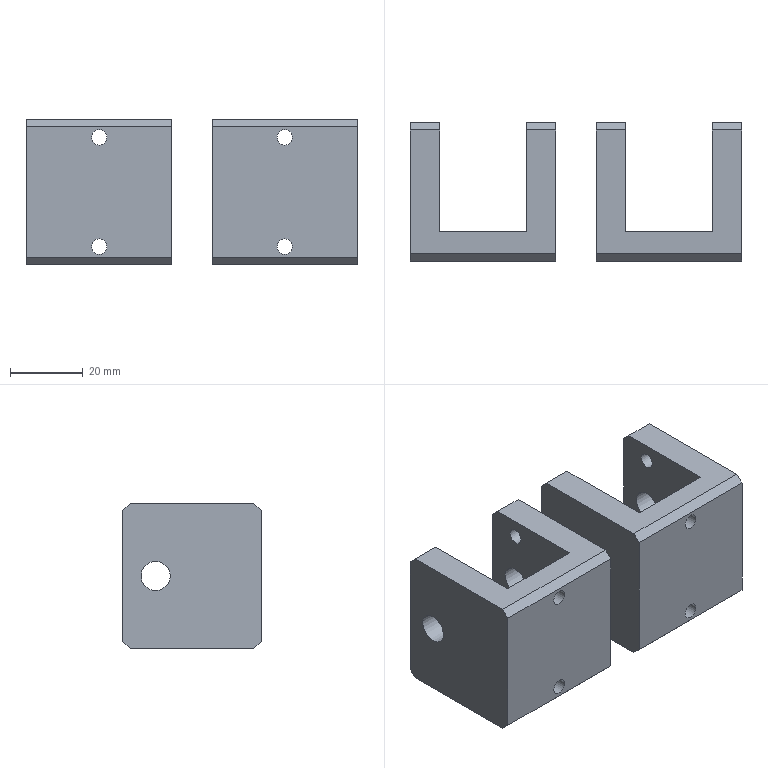NC program | NX | posted by the shop | part box 91 x 38 x 40 mm
Lines 3676 to 4199 of 4199:
N5 T10 M06
(D10-J  D=10. R=0. H=10 ce=0.30 di=0.00)
G00 G90 G54 X18.801 Y-28.3 M03 S6000
G43 H10 Z50.
M08
Z-29.5
G01 Z-30. F1200.
Y-25.
Y25.
X25.5
Y-25.
X32.2
Y25.
Y28.3
Z-29.5
G00 Z50.
X-32.199 Y-28.3
Z-29.5
G01 Z-30.
Y-25.
Y25.
X-25.5
Y-25.
X-18.8
Y25.
Y28.3
Z-29.5
G00 Z50.
G91 G28 Z0.0
M05
M09
G91 G28 Z0.0
M01
N6 T02 M06
(D6 chamfer mill  D=6. R=0. H=02 ce=0.00 di=0.00)
G00 G90 G54 X-46.707 Y-18.461 M03 S8000
G43 H02 Z50.
M08
Z2.935
G01 Z-1.5 F3000.
X-46.767 Y-18.289
X-46.8 Y-18.
Y18.
X-46.767 Y18.289
X-46.707 Y18.461
Z2.935
G00 Z3.45
X-36.293
Z2.935
G01 Z-1.5
X-36.233 Y18.289
X-36.2 Y18.
Y0.0
Y-18.
X-36.233 Y-18.289
X-36.293 Y-18.461
Z2.935
G00 Z50.
X-4.293 Y18.461
Z2.935
G01 Z-1.5
X-4.233 Y18.289
X-4.2 Y18.
Y-18.
X-4.233 Y-18.289
X-4.293 Y-18.461
Z2.935
G00 Z3.45
X-14.707
Z2.935
G01 Z-1.5
X-14.767 Y-18.289
X-14.8 Y-18.
Y0.0
Y18.
X-14.767 Y18.289
X-14.707 Y18.461
Z2.935
G00 Z50.
X14.707
Z2.935
G01 Z-1.5
X14.767 Y18.289
X14.8 Y18.
Y-18.
X14.767 Y-18.289
X14.707 Y-18.461
Z2.935
G00 Z3.45
X4.293
Z2.935
G01 Z-1.5
X4.233 Y-18.289
X4.2 Y-18.
Y0.0
Y18.
X4.233 Y18.289
X4.293 Y18.461
Z2.935
G00 Z50.
X46.707
Z2.935
G01 Z-1.5
X46.767 Y18.289
X46.8 Y18.
Y-18.
X46.767 Y-18.289
X46.707 Y-18.461
Z2.935
G00 Z3.45
X36.293
Z2.935
G01 Z-1.5
X36.233 Y-18.289
X36.2 Y-18.
Y0.0
Y18.
X36.233 Y18.289
X36.293 Y18.461
Z2.935
G00 Z50.
X34.468 Y-22.128
Z.567
G01 Z-31.5
G03 X34.549 Y-21.828 I-.52 J.3
X34.249 Y-21.308 I-.6 J0.0
G01 X34.219 Y-21.3
X16.781
X16.751 Y-21.308
G03 X16.451 Y-21.828 I.3 J-.52
X16.532 Y-22.128 I.6 J0.0
G01 Z.567
G00 Z50.
Y22.128
Z.567
G01 Z-31.5
G03 X16.451 Y21.828 I.52 J-.3
X16.751 Y21.308 I.6 J0.0
G01 X16.781 Y21.3
X34.219
X34.249 Y21.308
G03 X34.549 Y21.828 I-.3 J.52
X34.468 Y22.128 I-.6 J0.0
G01 Z.567
G00 Z50.
X-16.532 Y-22.128
Z.567
G01 Z-31.5
G03 X-16.451 Y-21.828 I-.52 J.3
X-16.751 Y-21.308 I-.6 J0.0
G01 X-16.781 Y-21.3
X-34.219
X-34.249 Y-21.308
G03 X-34.549 Y-21.828 I.3 J-.52
X-34.468 Y-22.128 I.6 J0.0
G01 Z.567
G00 Z50.
Y22.128
Z.567
G01 Z-31.5
G03 X-34.549 Y21.828 I.52 J-.3
X-34.249 Y21.308 I.6 J0.0
G01 X-34.219 Y21.3
X-16.781
X-16.751 Y21.308
G03 X-16.451 Y21.828 I-.3 J.52
X-16.532 Y22.128 I-.6 J0.0
G01 Z.567
G00 Z50.
G00 G90 X26.194 Y15.093 M03 S8000
Z50.
Z-30.5
G01 Z-31. F500.
X27. Y15.2
G03 X25.5 Y16.7 I-1.5 J0.0
X23.8 Y15. I0.0 J-1.7
X25.5 Y13.3 I1.7 J0.0
X27.2 Y15. I0.0 J1.7
X25.5 Y16.7 I-1.7 J0.0
X24. Y15.2 I0.0 J-1.5
G01 X24.806 Y15.093
Z-30.5
G00 Z50.
X26.194 Y-14.907
Z-30.5
G01 Z-31.
X27. Y-14.8
G03 X25.5 Y-13.3 I-1.5 J0.0
X23.8 Y-15. I0.0 J-1.7
X25.5 Y-16.7 I1.7 J0.0
X27.2 Y-15. I0.0 J1.7
X25.5 Y-13.3 I-1.7 J0.0
X24. Y-14.8 I0.0 J-1.5
G01 X24.806 Y-14.907
Z-30.5
G00 Z50.
X-24.806
Z-30.5
G01 Z-31.
X-24. Y-14.8
G03 X-25.5 Y-13.3 I-1.5 J0.0
X-27.2 Y-15. I0.0 J-1.7
X-25.5 Y-16.7 I1.7 J0.0
X-23.8 Y-15. I0.0 J1.7
X-25.5 Y-13.3 I-1.7 J0.0
X-27. Y-14.8 I0.0 J-1.5
G01 X-26.194 Y-14.907
Z-30.5
G00 Z50.
X-24.806 Y15.093
Z-30.5
G01 Z-31.
X-24. Y15.2
G03 X-25.5 Y16.7 I-1.5 J0.0
X-27.2 Y15. I0.0 J-1.7
X-25.5 Y13.3 I1.7 J0.0
X-23.8 Y15. I0.0 J1.7
X-25.5 Y16.7 I-1.7 J0.0
X-27. Y15.2 I0.0 J-1.5
G01 X-26.194 Y15.093
Z-30.5
G00 Z50.
G00 G90 X-33.6 Y-21.516 M03 S6500
Z50.
Z-1.2
G01 Z-2.7 F1000.
G03 X-34.737 Y-20.7 I-1.137 J-.384
G01 X-48.263
G03 X-49.4 Y-21.516 I0.0 J-1.2
G01 Z-1.2
G00 Z50.
Y21.516
Z-1.2
G01 Z-2.7
G03 X-48.263 Y20.7 I1.137 J.384
G01 X-34.737
G03 X-33.6 Y21.516 I0.0 J1.2
G01 Z-1.2
G00 Z50.
X-17.4
Z-1.2
G01 Z-2.7
G03 X-16.263 Y20.7 I1.137 J.384
G01 X-2.737
G03 X-1.6 Y21.516 I0.0 J1.2
G01 Z-1.2
G00 Z50.
X1.6
Z-1.2
G01 Z-2.7
G03 X2.737 Y20.7 I1.137 J.384
G01 X16.263
G03 X17.4 Y21.516 I0.0 J1.2
G01 Z-1.2
G00 Z50.
X-1.6 Y-21.516
Z-1.2
G01 Z-2.7
G03 X-2.737 Y-20.7 I-1.137 J-.384
G01 X-16.263
G03 X-17.4 Y-21.516 I0.0 J-1.2
G01 Z-1.2
G00 Z50.
X17.4
Z-1.2
G01 Z-2.7
G03 X16.263 Y-20.7 I-1.137 J-.384
G01 X2.737
G03 X1.6 Y-21.516 I0.0 J-1.2
G01 Z-1.2
G00 Z50.
X49.4
Z-1.2
G01 Z-2.7
G03 X48.263 Y-20.7 I-1.137 J-.384
G01 X34.737
G03 X33.6 Y-21.516 I0.0 J-1.2
G01 Z-1.2
G00 Z50.
Y21.516
Z-1.2
G01 Z-2.7
G03 X34.737 Y20.7 I1.137 J.384
G01 X48.263
G03 X49.4 Y21.516 I0.0 J1.2
G01 Z-1.2
G00 Z50.
G91 G28 Z0.0
M05
M09
G91 G28 Z0.0
M01
N7 T10 M06
(D10-J  D=10. R=0. H=10 ce=-0.03 di=0.01)
G00 G90 G54 X19.57 Y25.5 M03 S6000
G43 H10 Z50.
M08
Z-14.498
G01 Z-14.998 F1200.
G41 D10
X19.47
G03 X18.47 Y24.5 I0.0 J-1.
G01 Y-24.5
G03 X19.47 Y-25.5 I1. J0.0
G01 G40 X19.57
Z-14.498
G00 Z50.
X31.43
Z-14.498
G01 Z-14.998
G41 D10
X31.53
G03 X32.53 Y-24.5 I0.0 J1.
G01 Y24.5
G03 X31.53 Y25.5 I-1. J0.0
G01 G40 X31.43
Z-14.498
G00 Z50.
X19.57
Z-29.495
G01 Z-29.995
G41 D10
X19.47
G03 X18.47 Y24.5 I0.0 J-1.
G01 Y-24.5
G03 X19.47 Y-25.5 I1. J0.0
G01 G40 X19.57
X31.43
G41 D10
X31.53
G03 X32.53 Y-24.5 I0.0 J1.
G01 Y24.5
G03 X31.53 Y25.5 I-1. J0.0
G01 G40 X31.43
Z-29.495
G00 Z50.
X-31.43
Z-14.498
G01 Z-14.998
G41 D10
X-31.53
G03 X-32.53 Y24.5 I0.0 J-1.
G01 Y-24.5
G03 X-31.53 Y-25.5 I1. J0.0
G01 G40 X-31.43
Z-14.498
G00 Z50.
X-19.57
Z-14.498
G01 Z-14.998
G41 D10
X-19.47
G03 X-18.47 Y-24.5 I0.0 J1.
G01 Y24.5
G03 X-19.47 Y25.5 I-1. J0.0
G01 G40 X-19.57
Z-14.498
G00 Z50.
X-31.43
Z-29.495
G01 Z-29.995
G41 D10
X-31.53
G03 X-32.53 Y24.5 I0.0 J-1.
G01 Y-24.5
G03 X-31.53 Y-25.5 I1. J0.0
G01 G40 X-31.43
X-19.57
G41 D10
X-19.47
G03 X-18.47 Y-24.5 I0.0 J1.
G01 Y24.5
G03 X-19.47 Y25.5 I-1. J0.0
G01 G40 X-19.57
Z-29.495
G00 Z50.
G91 G28 Z0.0
M05
M09
G91 G28 Z0.0
M01
N8 T22 M06
(M5X0.8 D=4.2 DR_a=180 H=22)
G00 G90 G54 X25.5 Y15. M03 S500
G43 H22 Z20.
M08
G95
G98 G84 X25.5 Y15. Z-41.5 R-29. F.8 Q3.
Y-15.
X-25.5
Y15.
G80
G94
G00 Z20.
G91 G28 Z0.0
M05
M09
G91 G28 Z0.0
M01
N9 T10 M06
(D10-J  D=10. R=0. H=10 ce=-0.02 di=0.00)
G00 G90 G54 X-51.596 Y-21.013 M03 S8000
G43 H10 Z50.
M08
Z-12.167
G01 Z-12.667 F1000.
G41 D10
X-51.396 Y-20.996
G03 X-50.48 Y-20. I-.084 J.996
G01 Y20.
G02 X-45.5 Y24.98 I4.98 J0.0
G01 X-5.5
G02 X-.52 Y20. I0.0 J-4.98
G01 Y-20.
G02 X-5.5 Y-24.98 I-4.98 J0.0
G01 X-45.5
G02 X-50.48 Y-20. I0.0 J4.98
G01 Y-19.5
G03 X-51.48 Y-18.5 I-1. J0.0
G01 G40 X-51.68
Z-12.167
G00 Z50.
X26.5 Y-26.18
Z-12.167
G01 Z-12.667
G41 D10
Y-25.98
G03 X25.5 Y-24.98 I-1. J0.0
G01 X5.5
G02 X.52 Y-20. I0.0 J4.98
G01 Y20.
G02 X5.5 Y24.98 I4.98 J0.0
G01 X45.5
G02 X50.48 Y20. I0.0 J-4.98
G01 Y-20.
G02 X45.5 Y-24.98 I-4.98 J0.0
G01 X25.5
X25.
G03 X24. Y-25.98 I0.0 J-1.
G01 G40 Y-26.18
Z-12.167
G00 Z50.
X46.513 Y-26.096
Z-24.833
G01 Z-25.333
G41 D10
X46.496 Y-25.896
G03 X45.5 Y-24.98 I-.996 J-.084
G01 X5.5
G02 X.52 Y-20. I0.0 J4.98
G01 Y20.
G02 X5.5 Y24.98 I4.98 J0.0
G01 X45.5
G02 X50.48 Y20. I0.0 J-4.98
G01 Y-20.
G02 X45.5 Y-24.98 I-4.98 J0.0
G01 X45.
G03 X44. Y-25.98 I0.0 J-1.
G01 G40 Y-26.18
Z-24.833
G00 Z50.
X-24.5
Z-24.833
G01 Z-25.333
G41 D10
Y-25.98
G03 X-25.5 Y-24.98 I-1. J0.0
G01 X-45.5
G02 X-50.48 Y-20. I0.0 J4.98
G01 Y20.
G02 X-45.5 Y24.98 I4.98 J0.0
G01 X-5.5
G02 X-.52 Y20. I0.0 J-4.98
G01 Y-20.
G02 X-5.5 Y-24.98 I-4.98 J0.0
G01 X-25.5
X-26.
G03 X-27. Y-25.98 I0.0 J-1.
G01 G40 Y-26.18
Z-24.833
G00 Z50.
X-4.487 Y-26.096
Z-37.5
G01 Z-38.
G41 D10
X-4.504 Y-25.896
G03 X-5.5 Y-24.98 I-.996 J-.084
G01 X-45.5
G02 X-50.48 Y-20. I0.0 J4.98
G01 Y20.
G02 X-45.5 Y24.98 I4.98 J0.0
G01 X-5.5
G02 X-.52 Y20. I0.0 J-4.98
G01 Y-20.
G02 X-5.5 Y-24.98 I-4.98 J0.0
G01 X-6.
G03 X-7. Y-25.98 I0.0 J-1.
G01 G40 Y-26.18
X.365 Y-23.437
G41 D10
X.539 Y-23.34
G03 X1.052 Y-22.466 I-.487 J.873
X.963 Y-22.054 I-1. J0.0
G02 X.52 Y-20. I4.537 J2.054
G01 Y20.
G02 X5.5 Y24.98 I4.98 J0.0
G01 X45.5
G02 X50.48 Y20. I0.0 J-4.98
G01 Y-20.
G02 X45.5 Y-24.98 I-4.98 J0.0
G01 X5.5
G02 X.963 Y-22.054 I0.0 J4.98
X.78 Y-21.589 I4.537 J2.054
G03 X-.167 Y-20.908 I-.948 J-.319
X-.487 Y-20.96 I0.0 J-1.
G01 G40 X0.0 Y-22.347
Z-37.5
G00 Z50.
M05
M09
G91 G28 Z0.0
G91 G28 Y0.0
M30
%